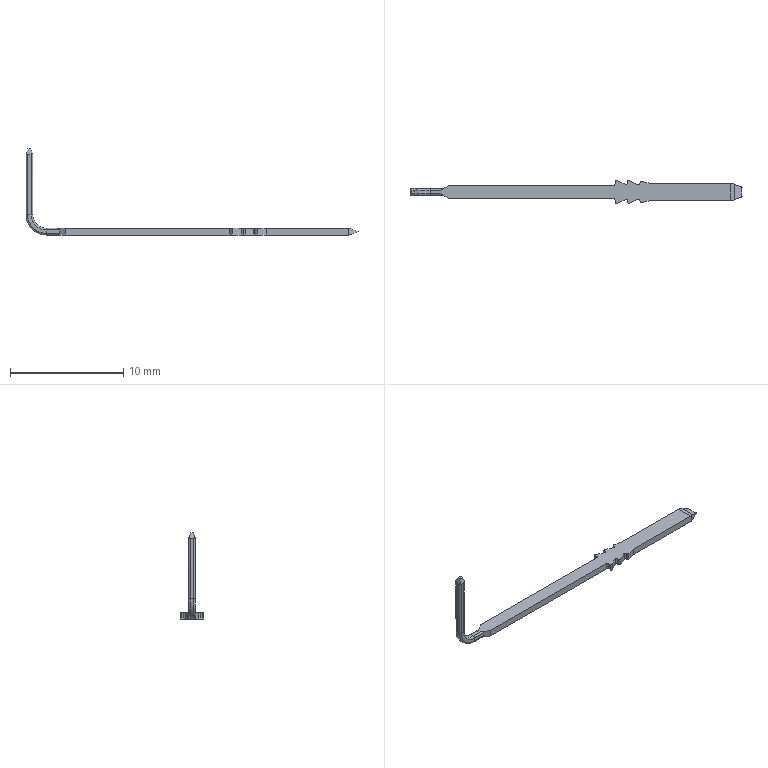Part | NX | features BREP 1 | 1 solid | 77 faces | box 29.3 x 2.1 x 7.6 mm | volume 23.902 mm3 | plane 38 | cylinder 35 | torus 2 | spline 2 | commonest cylinder face diameters 0.3 x16 0.2 x9 0.04 x4 0.025 x2 2 x2 2.4 x1